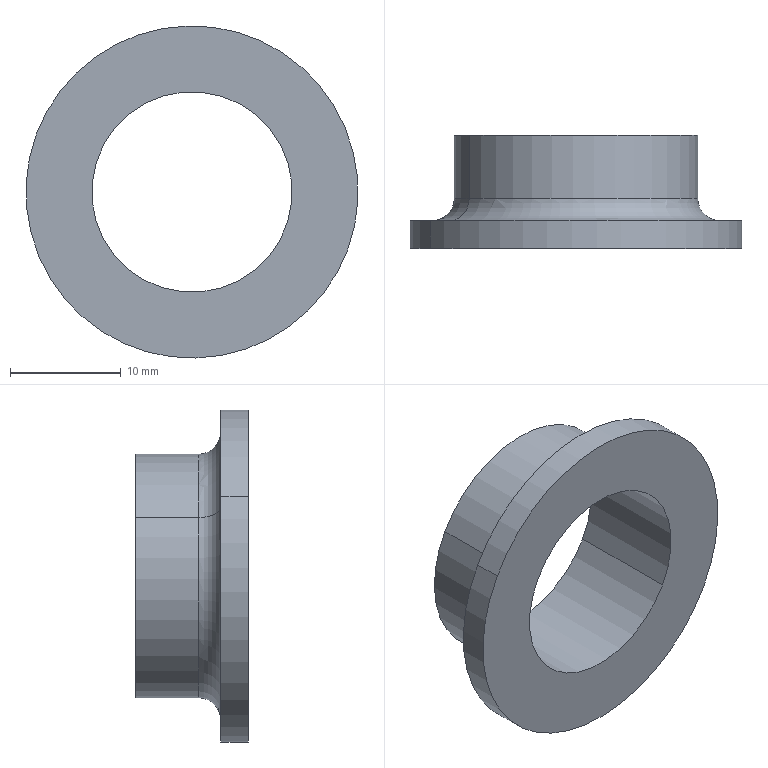Part | NX | features BREP 1 | 1 solid | 11 faces | box 30 x 10.2 x 30 mm | volume 2131 mm3 | cylinder 6 | plane 3 | torus 2 | commonest cylinder face diameters 18.1 x2 22 x2 30 x2
STEP:
#1=CARTESIAN_POINT('',(-291.857,-151.5,-146.148));
#2=VERTEX_POINT('',#1);
#3=CARTESIAN_POINT('',(-291.857,-154.,-146.148));
#4=VERTEX_POINT('',#3);
#5=CARTESIAN_POINT('',(-291.857,-151.5,-146.148));
#6=DIRECTION('',(0.,-1.,0.));
#7=VECTOR('',#6,1000.);
#8=LINE('',#5,#7);
#9=EDGE_CURVE('',#2,#4,#8,.T.);
#10=ORIENTED_EDGE('',*,*,#9,.T.);
#11=CARTESIAN_POINT('',(-265.529,-154.,-160.53));
#12=VERTEX_POINT('',#11);
#13=CARTESIAN_POINT('',(-278.693,-154.,-153.339));
#14=DIRECTION('',(0.,1.,0.));
#15=DIRECTION('',(-0.8776,0.,0.4794));
#16=AXIS2_PLACEMENT_3D('',#13,#14,#15);
#17=CIRCLE('',#16,15.);
#18=EDGE_CURVE('',#4,#12,#17,.T.);
#19=ORIENTED_EDGE('',*,*,#18,.T.);
#20=CARTESIAN_POINT('',(-265.529,-151.5,-160.53));
#21=VERTEX_POINT('',#20);
#22=CARTESIAN_POINT('',(-265.529,-151.5,-160.53));
#23=DIRECTION('',(0.,-1.,0.));
#24=VECTOR('',#23,1000.);
#25=LINE('',#22,#24);
#26=EDGE_CURVE('',#21,#12,#25,.T.);
#27=ORIENTED_EDGE('',*,*,#26,.F.);
#28=CARTESIAN_POINT('',(-278.693,-151.5,-153.339));
#29=DIRECTION('',(0.,1.,0.));
#30=DIRECTION('',(-0.8776,0.,0.4794));
#31=AXIS2_PLACEMENT_3D('',#28,#29,#30);
#32=CIRCLE('',#31,15.);
#33=EDGE_CURVE('',#2,#21,#32,.T.);
#34=ORIENTED_EDGE('',*,*,#33,.F.);
#35=EDGE_LOOP('',(#10,#19,#27,#34));
#36=FACE_BOUND('',#35,.T.);
#37=CARTESIAN_POINT('',(-278.693,-151.5,-153.339));
#38=DIRECTION('',(0.,-1.,0.));
#39=DIRECTION('',(0.8776,0.,-0.4794));
#40=AXIS2_PLACEMENT_3D('',#37,#38,#39);
#41=CYLINDRICAL_SURFACE('',#40,15.);
#42=ADVANCED_FACE('',(#36),#41,.T.);
#43=ORIENTED_EDGE('',*,*,#9,.F.);
#44=CARTESIAN_POINT('',(-278.693,-151.5,-153.339));
#45=DIRECTION('',(0.,1.,0.));
#46=DIRECTION('',(0.8776,0.,-0.4794));
#47=AXIS2_PLACEMENT_3D('',#44,#45,#46);
#48=CIRCLE('',#47,15.);
#49=EDGE_CURVE('',#21,#2,#48,.T.);
#50=ORIENTED_EDGE('',*,*,#49,.F.);
#51=ORIENTED_EDGE('',*,*,#26,.T.);
#52=CARTESIAN_POINT('',(-278.693,-154.,-153.339));
#53=DIRECTION('',(0.,1.,0.));
#54=DIRECTION('',(0.8776,0.,-0.4794));
#55=AXIS2_PLACEMENT_3D('',#52,#53,#54);
#56=CIRCLE('',#55,15.);
#57=EDGE_CURVE('',#12,#4,#56,.T.);
#58=ORIENTED_EDGE('',*,*,#57,.T.);
#59=EDGE_LOOP('',(#43,#50,#51,#58));
#60=FACE_BOUND('',#59,.T.);
#61=CARTESIAN_POINT('',(-278.693,-151.5,-153.339));
#62=DIRECTION('',(0.,-1.,0.));
#63=DIRECTION('',(0.8776,0.,-0.4794));
#64=AXIS2_PLACEMENT_3D('',#61,#62,#63);
#65=CYLINDRICAL_SURFACE('',#64,15.);
#66=ADVANCED_FACE('',(#60),#65,.T.);
#67=CARTESIAN_POINT('',(-286.635,-154.,-149.));
#68=VERTEX_POINT('',#67);
#69=CARTESIAN_POINT('',(-286.635,-143.8,-149.));
#70=VERTEX_POINT('',#69);
#71=CARTESIAN_POINT('',(-286.635,-154.,-149.));
#72=DIRECTION('',(0.,1.,0.));
#73=VECTOR('',#72,1000.);
#74=LINE('',#71,#73);
#75=EDGE_CURVE('',#68,#70,#74,.T.);
#76=ORIENTED_EDGE('',*,*,#75,.T.);
#77=CARTESIAN_POINT('',(-270.751,-143.8,-157.678));
#78=VERTEX_POINT('',#77);
#79=CARTESIAN_POINT('',(-278.693,-143.8,-153.339));
#80=DIRECTION('',(0.,1.,0.));
#81=DIRECTION('',(-0.8776,0.,0.4794));
#82=AXIS2_PLACEMENT_3D('',#79,#80,#81);
#83=CIRCLE('',#82,9.05);
#84=EDGE_CURVE('',#70,#78,#83,.T.);
#85=ORIENTED_EDGE('',*,*,#84,.T.);
#86=CARTESIAN_POINT('',(-270.751,-154.,-157.678));
#87=VERTEX_POINT('',#86);
#88=CARTESIAN_POINT('',(-270.751,-154.,-157.678));
#89=DIRECTION('',(0.,1.,0.));
#90=VECTOR('',#89,1000.);
#91=LINE('',#88,#90);
#92=EDGE_CURVE('',#87,#78,#91,.T.);
#93=ORIENTED_EDGE('',*,*,#92,.F.);
#94=CARTESIAN_POINT('',(-278.693,-154.,-153.339));
#95=DIRECTION('',(0.,1.,0.));
#96=DIRECTION('',(-0.8776,0.,0.4794));
#97=AXIS2_PLACEMENT_3D('',#94,#95,#96);
#98=CIRCLE('',#97,9.05);
#99=EDGE_CURVE('',#68,#87,#98,.T.);
#100=ORIENTED_EDGE('',*,*,#99,.F.);
#101=EDGE_LOOP('',(#76,#85,#93,#100));
#102=FACE_BOUND('',#101,.T.);
#103=CARTESIAN_POINT('',(-278.693,-154.,-153.339));
#104=DIRECTION('',(0.,1.,0.));
#105=DIRECTION('',(0.8776,0.,-0.4794));
#106=AXIS2_PLACEMENT_3D('',#103,#104,#105);
#107=CYLINDRICAL_SURFACE('',#106,9.05);
#108=ADVANCED_FACE('',(#102),#107,.F.);
#109=ORIENTED_EDGE('',*,*,#75,.F.);
#110=CARTESIAN_POINT('',(-278.693,-154.,-153.339));
#111=DIRECTION('',(0.,1.,0.));
#112=DIRECTION('',(0.8776,0.,-0.4794));
#113=AXIS2_PLACEMENT_3D('',#110,#111,#112);
#114=CIRCLE('',#113,9.05);
#115=EDGE_CURVE('',#87,#68,#114,.T.);
#116=ORIENTED_EDGE('',*,*,#115,.F.);
#117=ORIENTED_EDGE('',*,*,#92,.T.);
#118=CARTESIAN_POINT('',(-278.693,-143.8,-153.339));
#119=DIRECTION('',(0.,1.,0.));
#120=DIRECTION('',(0.8776,0.,-0.4794));
#121=AXIS2_PLACEMENT_3D('',#118,#119,#120);
#122=CIRCLE('',#121,9.05);
#123=EDGE_CURVE('',#78,#70,#122,.T.);
#124=ORIENTED_EDGE('',*,*,#123,.T.);
#125=EDGE_LOOP('',(#109,#116,#117,#124));
#126=FACE_BOUND('',#125,.T.);
#127=CARTESIAN_POINT('',(-278.693,-154.,-153.339));
#128=DIRECTION('',(0.,1.,0.));
#129=DIRECTION('',(0.8776,0.,-0.4794));
#130=AXIS2_PLACEMENT_3D('',#127,#128,#129);
#131=CYLINDRICAL_SURFACE('',#130,9.05);
#132=ADVANCED_FACE('',(#126),#131,.F.);
#133=CARTESIAN_POINT('',(-269.04,-143.8,-158.613));
#134=VERTEX_POINT('',#133);
#135=CARTESIAN_POINT('',(-288.346,-143.8,-148.065));
#136=VERTEX_POINT('',#135);
#137=CARTESIAN_POINT('',(-278.693,-143.8,-153.339));
#138=DIRECTION('',(0.,1.,0.));
#139=DIRECTION('',(0.8776,0.,-0.4794));
#140=AXIS2_PLACEMENT_3D('',#137,#138,#139);
#141=CIRCLE('',#140,11.);
#142=EDGE_CURVE('',#134,#136,#141,.T.);
#143=ORIENTED_EDGE('',*,*,#142,.T.);
#144=CARTESIAN_POINT('',(-278.693,-143.8,-153.339));
#145=DIRECTION('',(0.,1.,0.));
#146=DIRECTION('',(-0.8776,0.,0.4794));
#147=AXIS2_PLACEMENT_3D('',#144,#145,#146);
#148=CIRCLE('',#147,11.);
#149=EDGE_CURVE('',#136,#134,#148,.T.);
#150=ORIENTED_EDGE('',*,*,#149,.T.);
#151=EDGE_LOOP('',(#143,#150));
#152=FACE_BOUND('',#151,.T.);
#153=ORIENTED_EDGE('',*,*,#84,.F.);
#154=ORIENTED_EDGE('',*,*,#123,.F.);
#155=EDGE_LOOP('',(#153,#154));
#156=FACE_BOUND('',#155,.T.);
#157=CARTESIAN_POINT('',(-296.606,-143.8,-171.252));
#158=DIRECTION('',(0.,1.,0.));
#159=DIRECTION('',(-1.,0.,0.));
#160=AXIS2_PLACEMENT_3D('',#157,#158,#159);
#161=PLANE('',#160);
#162=ADVANCED_FACE('',(#152,#156),#161,.T.);
#163=ORIENTED_EDGE('',*,*,#57,.F.);
#164=ORIENTED_EDGE('',*,*,#18,.F.);
#165=EDGE_LOOP('',(#163,#164));
#166=FACE_BOUND('',#165,.T.);
#167=ORIENTED_EDGE('',*,*,#99,.T.);
#168=ORIENTED_EDGE('',*,*,#115,.T.);
#169=EDGE_LOOP('',(#167,#168));
#170=FACE_BOUND('',#169,.T.);
#171=CARTESIAN_POINT('',(-254.267,-154.,-128.913));
#172=DIRECTION('',(0.,-1.,0.));
#173=DIRECTION('',(0.,0.,1.));
#174=AXIS2_PLACEMENT_3D('',#171,#172,#173);
#175=PLANE('',#174);
#176=ADVANCED_FACE('',(#166,#170),#175,.T.);
#177=CARTESIAN_POINT('',(-288.346,-149.5,-148.065));
#178=VERTEX_POINT('',#177);
#179=CARTESIAN_POINT('',(-288.346,-143.8,-148.065));
#180=DIRECTION('',(0.,-1.,0.));
#181=VECTOR('',#180,1000.);
#182=LINE('',#179,#181);
#183=EDGE_CURVE('',#136,#178,#182,.T.);
#184=ORIENTED_EDGE('',*,*,#183,.T.);
#185=CARTESIAN_POINT('',(-269.04,-149.5,-158.613));
#186=VERTEX_POINT('',#185);
#187=CARTESIAN_POINT('',(-278.693,-149.5,-153.339));
#188=DIRECTION('',(0.,-1.,0.));
#189=DIRECTION('',(0.8776,0.,-0.4794));
#190=AXIS2_PLACEMENT_3D('',#187,#188,#189);
#191=CIRCLE('',#190,11.);
#192=EDGE_CURVE('',#186,#178,#191,.T.);
#193=ORIENTED_EDGE('',*,*,#192,.F.);
#194=CARTESIAN_POINT('',(-269.04,-143.8,-158.613));
#195=DIRECTION('',(0.,-1.,0.));
#196=VECTOR('',#195,1000.);
#197=LINE('',#194,#196);
#198=EDGE_CURVE('',#134,#186,#197,.T.);
#199=ORIENTED_EDGE('',*,*,#198,.F.);
#200=ORIENTED_EDGE('',*,*,#149,.F.);
#201=EDGE_LOOP('',(#184,#193,#199,#200));
#202=FACE_BOUND('',#201,.T.);
#203=CARTESIAN_POINT('',(-278.693,-143.8,-153.339));
#204=DIRECTION('',(0.,-1.,0.));
#205=DIRECTION('',(0.8776,0.,-0.4794));
#206=AXIS2_PLACEMENT_3D('',#203,#204,#205);
#207=CYLINDRICAL_SURFACE('',#206,11.);
#208=ADVANCED_FACE('',(#202),#207,.T.);
#209=ORIENTED_EDGE('',*,*,#183,.F.);
#210=ORIENTED_EDGE('',*,*,#142,.F.);
#211=ORIENTED_EDGE('',*,*,#198,.T.);
#212=CARTESIAN_POINT('',(-278.693,-149.5,-153.339));
#213=DIRECTION('',(0.,-1.,0.));
#214=DIRECTION('',(-0.8776,0.,0.4794));
#215=AXIS2_PLACEMENT_3D('',#212,#213,#214);
#216=CIRCLE('',#215,11.);
#217=EDGE_CURVE('',#178,#186,#216,.T.);
#218=ORIENTED_EDGE('',*,*,#217,.F.);
#219=EDGE_LOOP('',(#209,#210,#211,#218));
#220=FACE_BOUND('',#219,.T.);
#221=CARTESIAN_POINT('',(-278.693,-143.8,-153.339));
#222=DIRECTION('',(0.,-1.,0.));
#223=DIRECTION('',(0.8776,0.,-0.4794));
#224=AXIS2_PLACEMENT_3D('',#221,#222,#223);
#225=CYLINDRICAL_SURFACE('',#224,11.);
#226=ADVANCED_FACE('',(#220),#225,.T.);
#227=ORIENTED_EDGE('',*,*,#49,.T.);
#228=ORIENTED_EDGE('',*,*,#33,.T.);
#229=EDGE_LOOP('',(#227,#228));
#230=FACE_BOUND('',#229,.T.);
#231=CARTESIAN_POINT('',(-267.284,-151.5,-159.572));
#232=VERTEX_POINT('',#231);
#233=CARTESIAN_POINT('',(-290.102,-151.5,-147.106));
#234=VERTEX_POINT('',#233);
#235=CARTESIAN_POINT('',(-278.693,-151.5,-153.339));
#236=DIRECTION('',(0.,-1.,0.));
#237=DIRECTION('',(0.8776,0.,-0.4794));
#238=AXIS2_PLACEMENT_3D('',#235,#236,#237);
#239=CIRCLE('',#238,13.);
#240=EDGE_CURVE('',#232,#234,#239,.T.);
#241=ORIENTED_EDGE('',*,*,#240,.T.);
#242=CARTESIAN_POINT('',(-278.693,-151.5,-153.339));
#243=DIRECTION('',(0.,-1.,0.));
#244=DIRECTION('',(-0.8776,0.,0.4794));
#245=AXIS2_PLACEMENT_3D('',#242,#243,#244);
#246=CIRCLE('',#245,13.);
#247=EDGE_CURVE('',#234,#232,#246,.T.);
#248=ORIENTED_EDGE('',*,*,#247,.T.);
#249=EDGE_LOOP('',(#241,#248));
#250=FACE_BOUND('',#249,.T.);
#251=CARTESIAN_POINT('',(-303.119,-151.5,-177.765));
#252=DIRECTION('',(0.,1.,0.));
#253=DIRECTION('',(-1.,0.,0.));
#254=AXIS2_PLACEMENT_3D('',#251,#252,#253);
#255=PLANE('',#254);
#256=ADVANCED_FACE('',(#230,#250),#255,.T.);
#257=CARTESIAN_POINT('',(-290.102,-149.5,-147.106));
#258=DIRECTION('',(0.4794,0.,0.8776));
#259=DIRECTION('',(0.8776,0.,-0.4794));
#260=AXIS2_PLACEMENT_3D('',#257,#258,#259);
#261=CIRCLE('',#260,2.);
#262=EDGE_CURVE('',#234,#178,#261,.T.);
#263=ORIENTED_EDGE('',*,*,#262,.T.);
#264=ORIENTED_EDGE('',*,*,#217,.T.);
#265=CARTESIAN_POINT('',(-267.284,-149.5,-159.572));
#266=DIRECTION('',(-0.4794,0.,-0.8776));
#267=DIRECTION('',(-0.8776,0.,0.4794));
#268=AXIS2_PLACEMENT_3D('',#265,#266,#267);
#269=CIRCLE('',#268,2.);
#270=EDGE_CURVE('',#232,#186,#269,.T.);
#271=ORIENTED_EDGE('',*,*,#270,.F.);
#272=ORIENTED_EDGE('',*,*,#247,.F.);
#273=EDGE_LOOP('',(#263,#264,#271,#272));
#274=FACE_BOUND('',#273,.T.);
#275=CARTESIAN_POINT('',(-278.693,-149.5,-153.339));
#276=DIRECTION('',(0.,1.,0.));
#277=DIRECTION('',(-0.8776,0.,0.4794));
#278=AXIS2_PLACEMENT_3D('',#275,#276,#277);
#279=TOROIDAL_SURFACE('',#278,13.,2.);
#280=ADVANCED_FACE('',(#274),#279,.F.);
#281=ORIENTED_EDGE('',*,*,#270,.T.);
#282=ORIENTED_EDGE('',*,*,#192,.T.);
#283=ORIENTED_EDGE('',*,*,#262,.F.);
#284=ORIENTED_EDGE('',*,*,#240,.F.);
#285=EDGE_LOOP('',(#281,#282,#283,#284));
#286=FACE_BOUND('',#285,.T.);
#287=CARTESIAN_POINT('',(-278.693,-149.5,-153.339));
#288=DIRECTION('',(0.,1.,0.));
#289=DIRECTION('',(0.8776,0.,-0.4794));
#290=AXIS2_PLACEMENT_3D('',#287,#288,#289);
#291=TOROIDAL_SURFACE('',#290,13.,2.);
#292=ADVANCED_FACE('',(#286),#291,.F.);
#293=CLOSED_SHELL('',(#42,#66,#108,#132,#162,#176,#208,#226,#256,#280,#292));
#294=MANIFOLD_SOLID_BREP('',#293);
#295=(LENGTH_UNIT()NAMED_UNIT(*)SI_UNIT(.MILLI.,.METRE.));
#296=UNCERTAINTY_MEASURE_WITH_UNIT(LENGTH_MEASURE(0.00001),#295,'','');
#297=(NAMED_UNIT(*)PLANE_ANGLE_UNIT()SI_UNIT($,.RADIAN.));
#298=(NAMED_UNIT(*)SI_UNIT($,.STERADIAN.)SOLID_ANGLE_UNIT());
#299=(GEOMETRIC_REPRESENTATION_CONTEXT(3)GLOBAL_UNCERTAINTY_ASSIGNED_CONTEXT((#296))GLOBAL_UNIT_ASSIGNED_CONTEXT((#295,#297,#298))REPRESENTATION_CONTEXT('',''));
#300=ADVANCED_BREP_SHAPE_REPRESENTATION('',(#294),#299);